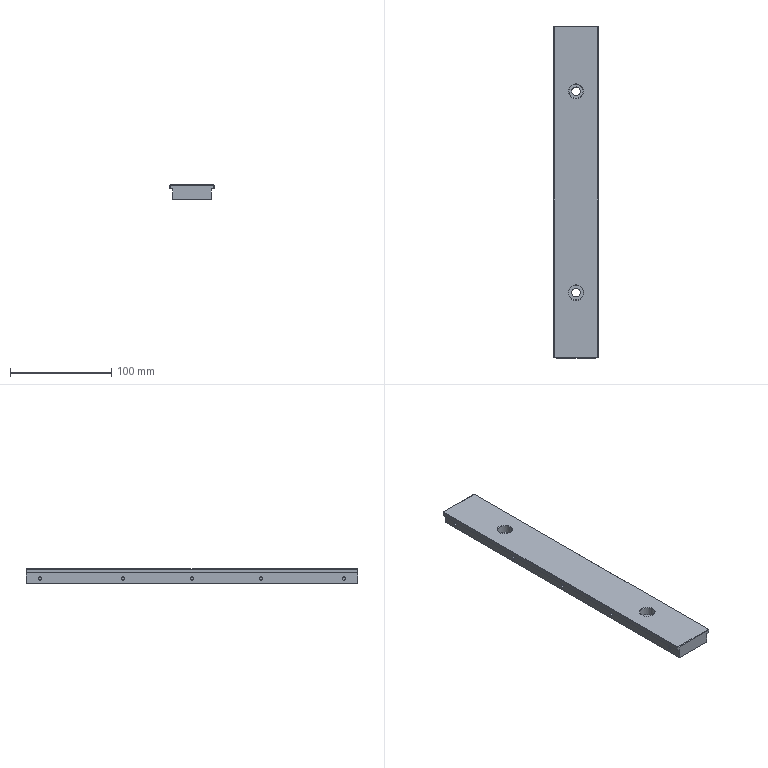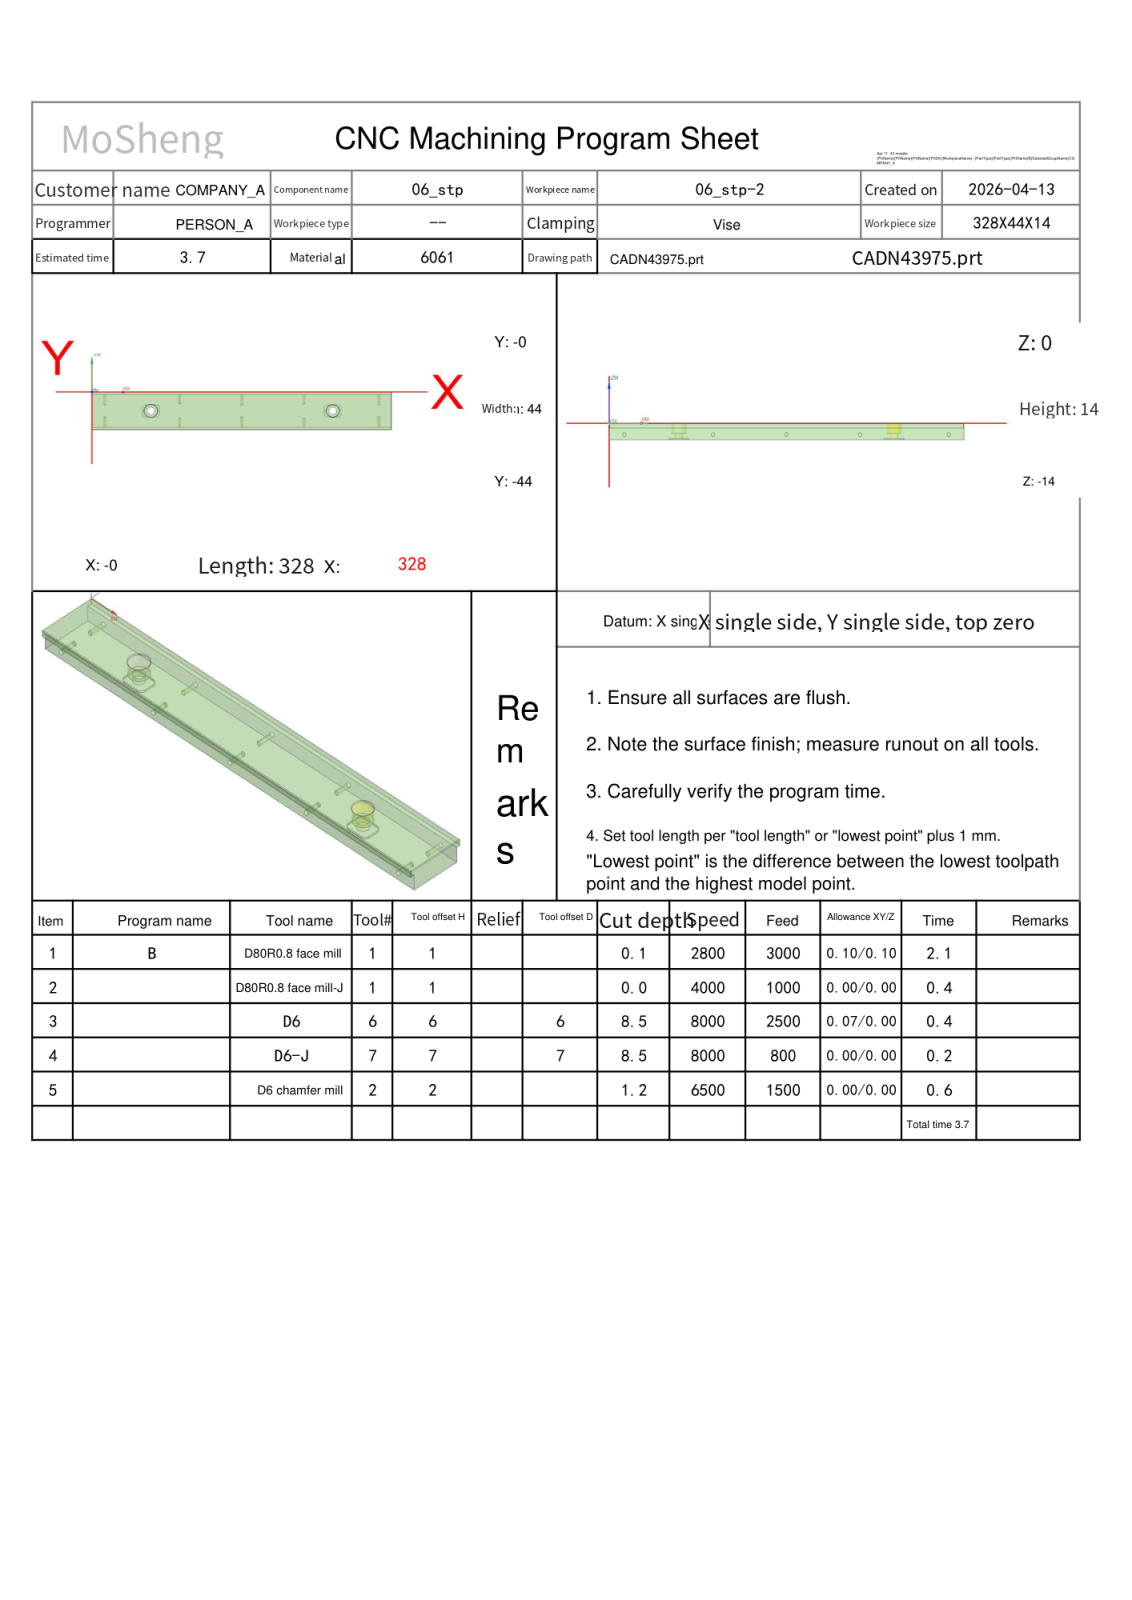NC program | NX | posted by the shop | part box 44 x 328 x 14 mm
Whole program:
%
O0001
(Machine time: 4.62 MIN)
(===Total Tool:4===)
(T1=D80R0.8 face mill D=80.  R=0.8  D-  H01 Z=-0.   )
(T6=D6      D=6.   R=0.   D6  H06 Z=-8.5  )
(T7=D6-J    D=6.   R=0.   D7  H07 Z=-8.5  )
(T2=D6 chamfer mill   D=6.   R=0.   D-  H02 Z=-1.2  )
G80 G90 G17 G49 G40
G91 G28 Z0
M01
N1 T01 M06
(D80R0.8 face mill  D=80. R=0.8 H=01 ce=0.10 di=0.10)
G00 G90 G54 X-52.097 Y-22. M03 S2800
G43 H01 Z20.
M08
Z7.009
G01 Z5.009 F3000.
X-40.097
X368.097
X380.097
Z7.009
G00 X-52.097
Z6.518
G01 Z4.518
X-40.097
X368.097
X380.097
Z6.518
G00 X-52.097
Z6.027
G01 Z4.027
X-40.097
X368.097
X380.097
Z6.027
G00 X-52.097
Z5.536
G01 Z3.536
X-40.097
X368.097
X380.097
Z5.536
G00 Z20.
X-52.097
Z5.045
G01 Z3.045
X-40.097
X368.097
X380.097
Z5.045
G00 Z20.
X-52.097
Z4.555
G01 Z2.555
X-40.097
X368.097
X380.097
Z4.555
G00 Z20.
X-52.097
Z4.064
G01 Z2.064
X-40.097
X368.097
X380.097
Z4.064
G00 Z20.
X-52.097
Z3.573
G01 Z1.573
X-40.097
X368.097
X380.097
Z3.573
G00 Z20.
X-52.097
Z3.082
G01 Z1.082
X-40.097
X368.097
X380.097
Z3.082
G00 Z20.
X-52.097
Z2.591
G01 Z.591
X-40.097
X368.097
X380.097
Z2.591
G00 Z20.
X-52.097
Z2.1
G01 Z.1
X-40.097
X368.097
X380.097
Z2.1
G00 Z20.
G91 G28 Z0.0
M05
M09
G91 G28 Z0.0
M01
N2 T01 M06
(D80R0.8 face mill-J  D=80. R=0.8 H=01 ce=0.00 di=0.00)
G00 G90 G54 X-51.999 Y-22. M03 S4000
G43 H01 Z20.
M08
Z2.
G01 Z0.0 F1000.
X-39.999
X367.999
X379.999
Z2.
G00 Z20.
G91 G28 Z0.0
M05
M09
G91 G28 Z0.0
M01
N3 T06 M06
(D6  D=6. R=0. H=06 ce=0.07 di=0.00)
G00 G90 G54 X263.5 Y-22. M03 S8000
G43 H06 Z20.
M08
Z.8
G41 D06
G01 X263.4 Y-22.005 F2500.
G03 X261.536 Y-23.966 I.1 J-1.961
X263.5 Y-25.93 I1.964 J0.0
X263.5 Y-25.93 Z.3 I0.0 J3.93
X263.5 Y-25.93 Z-.2 I0.0 J3.93
X263.5 Y-25.93 Z-.7 I0.0 J3.93
X263.5 Y-25.93 Z-1.2 I0.0 J3.93
X263.5 Y-25.93 Z-1.7 I0.0 J3.93
X263.5 Y-25.93 Z-2.2 I0.0 J3.93
X263.5 Y-25.93 Z-2.7 I0.0 J3.93
X263.5 Y-25.93 Z-3.2 I0.0 J3.93
X263.5 Y-25.93 Z-3.7 I0.0 J3.93
X263.5 Y-25.93 Z-4.2 I0.0 J3.93
X263.5 Y-25.93 Z-4.7 I0.0 J3.93
X263.5 Y-25.93 Z-5.2 I0.0 J3.93
X263.5 Y-25.93 Z-5.7 I0.0 J3.93
X263.5 Y-25.93 Z-6.2 I0.0 J3.93
X263.5 Y-25.93 Z-6.7 I0.0 J3.93
X263.5 Y-25.93 Z-7.2 I0.0 J3.93
X263.5 Y-25.93 Z-7.7 I0.0 J3.93
X263.5 Y-25.93 Z-8.2 I0.0 J3.93
X261.19 Y-18.821 Z-8.5 I0.0 J3.93
X259.57 Y-22. I2.31 J-3.179
X263.5 Y-25.93 I3.93 J0.0
X267.43 Y-22. I0.0 J3.93
X263.5 Y-18.07 I-3.93 J0.0
X261.19 Y-18.821 I0.0 J-3.93
X260.381 Y-20.409 I1.154 J-1.589
X262.344 Y-22.373 I1.964 J0.0
X263.416 Y-22.055 I0.0 J1.964
G01 G40 X263.5 Y-22.
G00 Z20.
G00 G90 X64.5 Y-22. M03 S8000
Z20.
Z.8
G41 D06
G01 X64.4 Y-22.005 F2500.
G03 X62.411 Y-24.091 I.1 J-2.086
X64.5 Y-26.18 I2.089 J0.0
X64.5 Y-26.18 Z.3 I0.0 J4.18
X64.5 Y-26.18 Z-.2 I0.0 J4.18
X64.5 Y-26.18 Z-.7 I0.0 J4.18
X64.5 Y-26.18 Z-1.2 I0.0 J4.18
X64.5 Y-26.18 Z-1.7 I0.0 J4.18
X64.5 Y-26.18 Z-2.2 I0.0 J4.18
X64.5 Y-26.18 Z-2.7 I0.0 J4.18
X64.5 Y-26.18 Z-3.2 I0.0 J4.18
X64.5 Y-26.18 Z-3.7 I0.0 J4.18
X64.5 Y-26.18 Z-4.2 I0.0 J4.18
X64.5 Y-26.18 Z-4.7 I0.0 J4.18
X64.5 Y-26.18 Z-5.2 I0.0 J4.18
X64.5 Y-26.18 Z-5.7 I0.0 J4.18
X64.5 Y-26.18 Z-6.2 I0.0 J4.18
X64.5 Y-26.18 Z-6.7 I0.0 J4.18
X64.5 Y-26.18 Z-7.2 I0.0 J4.18
X64.5 Y-26.18 Z-7.7 I0.0 J4.18
X64.5 Y-26.18 Z-8.2 I0.0 J4.18
X62.043 Y-18.618 Z-8.5 I0.0 J4.18
X60.32 Y-22. I2.457 J-3.382
X64.5 Y-26.18 I4.18 J0.0
X68.68 Y-22. I0.0 J4.18
X64.5 Y-17.82 I-4.18 J0.0
X62.043 Y-18.618 I0.0 J-4.18
X61.182 Y-20.308 I1.228 J-1.69
X63.271 Y-22.397 I2.089 J0.0
X64.416 Y-22.055 I0.0 J2.089
G01 G40 X64.5 Y-22.
G00 Z20.
G91 G28 Z0.0
M05
M09
G91 G28 Z0.0
M01
N4 T07 M06
(D6-J  D=6. R=0. H=07 ce=0.00 di=0.00)
G00 G90 G54 X263.5 Y-22. M03 S8000
G43 H07 Z20.
M08
Z-4.
G41 D07
G01 X263.149 Y-25.613 F800.
X263.147 Y-25.647
G03 X263.5 Y-26. I.353 J0.0
X267.5 Y-22. I0.0 J4.
X263.5 Y-18. I-4. J0.0
X259.5 Y-22. I0.0 J-4.
X263.5 Y-26. I4. J0.0
X263.999 Y-25.969 I0.0 J4.
X264.308 Y-25.619 I-.044 J.35
G01 X264.299 Y-25.541
G40 X263.5 Y-22.
Z-8.5 F10000.
G41 D07
X263.149 Y-25.613 F800.
X263.147 Y-25.647
G03 X263.5 Y-26. I.353 J0.0
X267.5 Y-22. I0.0 J4.
X263.5 Y-18. I-4. J0.0
X259.5 Y-22. I0.0 J-4.
X263.5 Y-26. I4. J0.0
X263.999 Y-25.969 I0.0 J4.
X264.308 Y-25.619 I-.044 J.35
G01 X264.299 Y-25.541
G40 X263.5 Y-22.
G00 Z20.
G00 G90 X64.5 Y-22. M03 S8000
Z20.
Z-4.
G41 D07
G01 X64.148 Y-25.864 F800.
X64.146 Y-25.896
G03 X64.5 Y-26.25 I.354 J0.0
X68.75 Y-22. I0.0 J4.25
X64.5 Y-17.75 I-4.25 J0.0
X60.25 Y-22. I0.0 J-4.25
X64.5 Y-26.25 I4.25 J0.0
X64.999 Y-26.221 I0.0 J4.25
X65.311 Y-25.869 I-.042 J.351
G01 X65.304 Y-25.796
G40 X64.5 Y-22.
Z-8.5 F10000.
G41 D07
X64.148 Y-25.864 F800.
X64.146 Y-25.896
G03 X64.5 Y-26.25 I.354 J0.0
X68.75 Y-22. I0.0 J4.25
X64.5 Y-17.75 I-4.25 J0.0
X60.25 Y-22. I0.0 J-4.25
X64.5 Y-26.25 I4.25 J0.0
X64.999 Y-26.221 I0.0 J4.25
X65.311 Y-25.869 I-.042 J.351
G01 X65.304 Y-25.796
G40 X64.5 Y-22.
G00 Z20.
G91 G28 Z0.0
M05
M09
G91 G28 Z0.0
M01
N5 T02 M06
(D6 chamfer mill  D=6. R=0. H=02 ce=0.00 di=0.00)
G00 G90 G54 X65.7 Y-16.786 M03 S6500
G43 H02 Z20.
M08
Z.3
G01 Z-1.2 F1500.
Y-16.65
G03 X64.5 Y-15.45 I-1.2 J0.0
X57.95 Y-22. I0.0 J-6.55
X64.5 Y-28.55 I6.55 J0.0
X71.05 Y-22. I0.0 J6.55
X64.5 Y-15.45 I-6.55 J0.0
X64.1 Y-15.462 I0.0 J-6.55
X62.973 Y-16.66 I.073 J-1.198
G01 X62.976 Y-16.733
X62.984 Y-16.869
Z.3
G00 Z20.
X-.85 Y1.337
Z.3
G01 Z-1.2
G03 X.21 Y.7 I1.06 J.563
G01 X327.79
X328.7 Y-.21
Y-43.79
X327.79 Y-44.7
X.21
X-.7 Y-43.79
Y-.21
X.21 Y.7
X.61
G03 X1.81 Y1.9 I0.0 J1.2
G01 Z.3
G00 Z20.
X264.7 Y-17.043
Z.3
G01 Z-1.2
Y-16.9
G03 X263.5 Y-15.7 I-1.2 J0.0
X257.2 Y-22. I0.0 J-6.3
X263.5 Y-28.3 I6.3 J0.0
X269.8 Y-22. I0.0 J6.3
X263.5 Y-15.7 I-6.3 J0.0
X263.1 Y-15.713 I0.0 J-6.3
X261.976 Y-16.91 I.076 J-1.198
G01 X261.979 Y-16.986
X261.988 Y-17.129
Z.3
G00 Z20.
M05
M09
G91 G28 Z0.0
G91 G28 Y0.0
M30
%